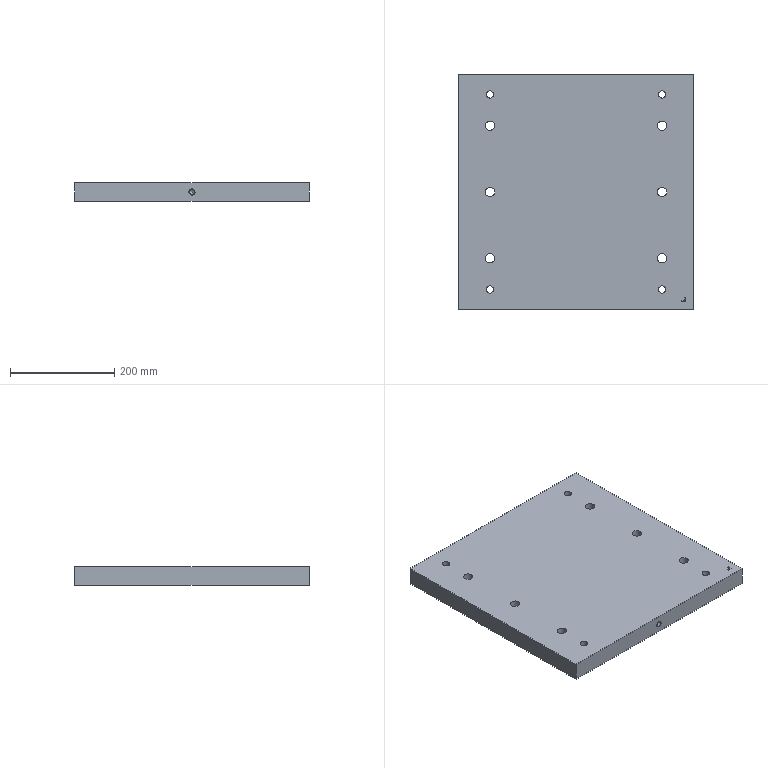Part | NX | features solid 2 | 1 solid | 59 faces | box 450 x 450 x 35 mm | volume 6967341 mm3 | plane 31 | cylinder 26 | cone 2 | commonest cylinder face diameters 18 x6 26 x6 14 x4 20 x4 10.2 x2 11.7 x2
STEP:
#1=CARTESIAN_POINT('',(0.,225.,-392.9));
#2=VERTEX_POINT('',#1);
#3=CARTESIAN_POINT('',(0.,225.,-398.));
#4=DIRECTION('',(0.,1.,0.));
#5=DIRECTION('',(0.,0.,1.));
#6=AXIS2_PLACEMENT_3D('',#3,#4,#5);
#7=CIRCLE('',#6,5.1);
#8=EDGE_CURVE('',#2,#2,#7,.T.);
#9=ORIENTED_EDGE('',*,*,#8,.F.);
#10=EDGE_LOOP('',(#9));
#11=FACE_BOUND('',#10,.T.);
#12=CARTESIAN_POINT('',(-225.,225.,-415.5));
#13=VERTEX_POINT('',#12);
#14=CARTESIAN_POINT('',(-225.,225.,-380.5));
#15=VERTEX_POINT('',#14);
#16=CARTESIAN_POINT('',(-225.,225.,-415.5));
#17=DIRECTION('',(0.,0.,1.));
#18=VECTOR('',#17,1000.);
#19=LINE('',#16,#18);
#20=EDGE_CURVE('',#13,#15,#19,.T.);
#21=ORIENTED_EDGE('',*,*,#20,.T.);
#22=CARTESIAN_POINT('',(225.,225.,-380.5));
#23=VERTEX_POINT('',#22);
#24=CARTESIAN_POINT('',(0.,225.,-380.5));
#25=DIRECTION('',(1.,0.,0.));
#26=VECTOR('',#25,1000.);
#27=LINE('',#24,#26);
#28=EDGE_CURVE('',#15,#23,#27,.T.);
#29=ORIENTED_EDGE('',*,*,#28,.T.);
#30=CARTESIAN_POINT('',(225.,225.,-415.5));
#31=VERTEX_POINT('',#30);
#32=CARTESIAN_POINT('',(225.,225.,-415.5));
#33=DIRECTION('',(0.,0.,1.));
#34=VECTOR('',#33,1000.);
#35=LINE('',#32,#34);
#36=EDGE_CURVE('',#31,#23,#35,.T.);
#37=ORIENTED_EDGE('',*,*,#36,.F.);
#38=CARTESIAN_POINT('',(0.,225.,-415.5));
#39=DIRECTION('',(-1.,0.,0.));
#40=VECTOR('',#39,1000.);
#41=LINE('',#38,#40);
#42=EDGE_CURVE('',#31,#13,#41,.T.);
#43=ORIENTED_EDGE('',*,*,#42,.T.);
#44=EDGE_LOOP('',(#21,#29,#37,#43));
#45=FACE_BOUND('',#44,.T.);
#46=CARTESIAN_POINT('',(0.,225.,-403.85));
#47=VERTEX_POINT('',#46);
#48=CARTESIAN_POINT('',(5.85,225.,-398.));
#49=VERTEX_POINT('',#48);
#50=CARTESIAN_POINT('',(0.,225.,-398.));
#51=DIRECTION('',(0.,1.,0.));
#52=DIRECTION('',(0.,0.,1.));
#53=AXIS2_PLACEMENT_3D('',#50,#51,#52);
#54=CIRCLE('',#53,5.85);
#55=EDGE_CURVE('',#47,#49,#54,.T.);
#56=ORIENTED_EDGE('',*,*,#55,.T.);
#57=CARTESIAN_POINT('',(6.,225.,-398.));
#58=VERTEX_POINT('',#57);
#59=CARTESIAN_POINT('',(0.,225.,-398.));
#60=DIRECTION('',(1.,0.,0.));
#61=VECTOR('',#60,1000.);
#62=LINE('',#59,#61);
#63=EDGE_CURVE('',#49,#58,#62,.T.);
#64=ORIENTED_EDGE('',*,*,#63,.T.);
#65=CARTESIAN_POINT('',(0.,225.,-404.));
#66=VERTEX_POINT('',#65);
#67=CARTESIAN_POINT('',(0.,225.,-398.));
#68=DIRECTION('',(0.,1.,0.));
#69=DIRECTION('',(0.,0.,1.));
#70=AXIS2_PLACEMENT_3D('',#67,#68,#69);
#71=CIRCLE('',#70,6.);
#72=EDGE_CURVE('',#66,#58,#71,.T.);
#73=ORIENTED_EDGE('',*,*,#72,.F.);
#74=CARTESIAN_POINT('',(0.,225.,-415.5));
#75=DIRECTION('',(0.,0.,1.));
#76=VECTOR('',#75,1000.);
#77=LINE('',#74,#76);
#78=EDGE_CURVE('',#66,#47,#77,.T.);
#79=ORIENTED_EDGE('',*,*,#78,.T.);
#80=EDGE_LOOP('',(#56,#64,#73,#79));
#81=FACE_BOUND('',#80,.T.);
#82=CARTESIAN_POINT('',(0.,225.,-415.5));
#83=DIRECTION('',(0.,1.,0.));
#84=DIRECTION('',(0.,0.,1.));
#85=AXIS2_PLACEMENT_3D('',#82,#83,#84);
#86=PLANE('',#85);
#87=ADVANCED_FACE('',(#11,#45,#81),#86,.T.);
#88=CARTESIAN_POINT('',(0.,-225.,-403.1));
#89=VERTEX_POINT('',#88);
#90=CARTESIAN_POINT('',(0.,-225.,-398.));
#91=DIRECTION('',(0.,-1.,0.));
#92=DIRECTION('',(0.,0.,-1.));
#93=AXIS2_PLACEMENT_3D('',#90,#91,#92);
#94=CIRCLE('',#93,5.1);
#95=EDGE_CURVE('',#89,#89,#94,.T.);
#96=ORIENTED_EDGE('',*,*,#95,.F.);
#97=EDGE_LOOP('',(#96));
#98=FACE_BOUND('',#97,.T.);
#99=CARTESIAN_POINT('',(225.,-225.,-415.5));
#100=VERTEX_POINT('',#99);
#101=CARTESIAN_POINT('',(225.,-225.,-380.5));
#102=VERTEX_POINT('',#101);
#103=CARTESIAN_POINT('',(225.,-225.,-415.5));
#104=DIRECTION('',(0.,0.,1.));
#105=VECTOR('',#104,1000.);
#106=LINE('',#103,#105);
#107=EDGE_CURVE('',#100,#102,#106,.T.);
#108=ORIENTED_EDGE('',*,*,#107,.T.);
#109=CARTESIAN_POINT('',(-225.,-225.,-380.5));
#110=VERTEX_POINT('',#109);
#111=CARTESIAN_POINT('',(0.,-225.,-380.5));
#112=DIRECTION('',(-1.,0.,0.));
#113=VECTOR('',#112,1000.);
#114=LINE('',#111,#113);
#115=EDGE_CURVE('',#102,#110,#114,.T.);
#116=ORIENTED_EDGE('',*,*,#115,.T.);
#117=CARTESIAN_POINT('',(-225.,-225.,-415.5));
#118=VERTEX_POINT('',#117);
#119=CARTESIAN_POINT('',(-225.,-225.,-415.5));
#120=DIRECTION('',(0.,0.,1.));
#121=VECTOR('',#120,1000.);
#122=LINE('',#119,#121);
#123=EDGE_CURVE('',#118,#110,#122,.T.);
#124=ORIENTED_EDGE('',*,*,#123,.F.);
#125=CARTESIAN_POINT('',(0.,-225.,-415.5));
#126=DIRECTION('',(1.,0.,0.));
#127=VECTOR('',#126,1000.);
#128=LINE('',#125,#127);
#129=EDGE_CURVE('',#118,#100,#128,.T.);
#130=ORIENTED_EDGE('',*,*,#129,.T.);
#131=EDGE_LOOP('',(#108,#116,#124,#130));
#132=FACE_BOUND('',#131,.T.);
#133=CARTESIAN_POINT('',(0.,-225.,-392.15));
#134=VERTEX_POINT('',#133);
#135=CARTESIAN_POINT('',(5.85,-225.,-398.));
#136=VERTEX_POINT('',#135);
#137=CARTESIAN_POINT('',(0.,-225.,-398.));
#138=DIRECTION('',(0.,-1.,0.));
#139=DIRECTION('',(0.,0.,-1.));
#140=AXIS2_PLACEMENT_3D('',#137,#138,#139);
#141=CIRCLE('',#140,5.85);
#142=EDGE_CURVE('',#134,#136,#141,.T.);
#143=ORIENTED_EDGE('',*,*,#142,.T.);
#144=CARTESIAN_POINT('',(6.,-225.,-398.));
#145=VERTEX_POINT('',#144);
#146=CARTESIAN_POINT('',(0.,-225.,-398.));
#147=DIRECTION('',(1.,0.,0.));
#148=VECTOR('',#147,1000.);
#149=LINE('',#146,#148);
#150=EDGE_CURVE('',#136,#145,#149,.T.);
#151=ORIENTED_EDGE('',*,*,#150,.T.);
#152=CARTESIAN_POINT('',(0.,-225.,-392.));
#153=VERTEX_POINT('',#152);
#154=CARTESIAN_POINT('',(0.,-225.,-398.));
#155=DIRECTION('',(0.,-1.,0.));
#156=DIRECTION('',(0.,0.,-1.));
#157=AXIS2_PLACEMENT_3D('',#154,#155,#156);
#158=CIRCLE('',#157,6.);
#159=EDGE_CURVE('',#153,#145,#158,.T.);
#160=ORIENTED_EDGE('',*,*,#159,.F.);
#161=CARTESIAN_POINT('',(0.,-225.,-415.5));
#162=DIRECTION('',(0.,0.,-1.));
#163=VECTOR('',#162,1000.);
#164=LINE('',#161,#163);
#165=EDGE_CURVE('',#153,#134,#164,.T.);
#166=ORIENTED_EDGE('',*,*,#165,.T.);
#167=EDGE_LOOP('',(#143,#151,#160,#166));
#168=FACE_BOUND('',#167,.T.);
#169=CARTESIAN_POINT('',(0.,-225.,-415.5));
#170=DIRECTION('',(0.,-1.,0.));
#171=DIRECTION('',(0.,0.,-1.));
#172=AXIS2_PLACEMENT_3D('',#169,#170,#171);
#173=PLANE('',#172);
#174=ADVANCED_FACE('',(#98,#132,#168),#173,.T.);
#175=CARTESIAN_POINT('',(-156.,127.,-380.5));
#176=VERTEX_POINT('',#175);
#177=CARTESIAN_POINT('',(-165.,127.,-380.5));
#178=DIRECTION('',(0.,0.,1.));
#179=DIRECTION('',(1.,0.,0.));
#180=AXIS2_PLACEMENT_3D('',#177,#178,#179);
#181=CIRCLE('',#180,9.);
#182=EDGE_CURVE('',#176,#176,#181,.T.);
#183=ORIENTED_EDGE('',*,*,#182,.F.);
#184=EDGE_LOOP('',(#183));
#185=FACE_BOUND('',#184,.T.);
#186=CARTESIAN_POINT('',(-156.,0.,-380.5));
#187=VERTEX_POINT('',#186);
#188=CARTESIAN_POINT('',(-165.,0.,-380.5));
#189=DIRECTION('',(0.,0.,1.));
#190=DIRECTION('',(1.,0.,0.));
#191=AXIS2_PLACEMENT_3D('',#188,#189,#190);
#192=CIRCLE('',#191,9.);
#193=EDGE_CURVE('',#187,#187,#192,.T.);
#194=ORIENTED_EDGE('',*,*,#193,.F.);
#195=EDGE_LOOP('',(#194));
#196=FACE_BOUND('',#195,.T.);
#197=CARTESIAN_POINT('',(-156.,-127.,-380.5));
#198=VERTEX_POINT('',#197);
#199=CARTESIAN_POINT('',(-165.,-127.,-380.5));
#200=DIRECTION('',(0.,0.,1.));
#201=DIRECTION('',(1.,0.,0.));
#202=AXIS2_PLACEMENT_3D('',#199,#200,#201);
#203=CIRCLE('',#202,9.);
#204=EDGE_CURVE('',#198,#198,#203,.T.);
#205=ORIENTED_EDGE('',*,*,#204,.F.);
#206=EDGE_LOOP('',(#205));
#207=FACE_BOUND('',#206,.T.);
#208=CARTESIAN_POINT('',(174.,-127.,-380.5));
#209=VERTEX_POINT('',#208);
#210=CARTESIAN_POINT('',(165.,-127.,-380.5));
#211=DIRECTION('',(0.,0.,1.));
#212=DIRECTION('',(1.,0.,0.));
#213=AXIS2_PLACEMENT_3D('',#210,#211,#212);
#214=CIRCLE('',#213,9.);
#215=EDGE_CURVE('',#209,#209,#214,.T.);
#216=ORIENTED_EDGE('',*,*,#215,.F.);
#217=EDGE_LOOP('',(#216));
#218=FACE_BOUND('',#217,.T.);
#219=CARTESIAN_POINT('',(174.,0.,-380.5));
#220=VERTEX_POINT('',#219);
#221=CARTESIAN_POINT('',(165.,0.,-380.5));
#222=DIRECTION('',(0.,0.,1.));
#223=DIRECTION('',(1.,0.,0.));
#224=AXIS2_PLACEMENT_3D('',#221,#222,#223);
#225=CIRCLE('',#224,9.);
#226=EDGE_CURVE('',#220,#220,#225,.T.);
#227=ORIENTED_EDGE('',*,*,#226,.F.);
#228=EDGE_LOOP('',(#227));
#229=FACE_BOUND('',#228,.T.);
#230=CARTESIAN_POINT('',(174.,127.,-380.5));
#231=VERTEX_POINT('',#230);
#232=CARTESIAN_POINT('',(165.,127.,-380.5));
#233=DIRECTION('',(0.,0.,1.));
#234=DIRECTION('',(1.,0.,0.));
#235=AXIS2_PLACEMENT_3D('',#232,#233,#234);
#236=CIRCLE('',#235,9.);
#237=EDGE_CURVE('',#231,#231,#236,.T.);
#238=ORIENTED_EDGE('',*,*,#237,.F.);
#239=EDGE_LOOP('',(#238));
#240=FACE_BOUND('',#239,.T.);
#241=CARTESIAN_POINT('',(-158.,187.,-380.5));
#242=VERTEX_POINT('',#241);
#243=CARTESIAN_POINT('',(-165.,187.,-380.5));
#244=DIRECTION('',(0.,0.,-1.));
#245=DIRECTION('',(1.,0.,0.));
#246=AXIS2_PLACEMENT_3D('',#243,#244,#245);
#247=CIRCLE('',#246,7.);
#248=EDGE_CURVE('',#242,#242,#247,.T.);
#249=ORIENTED_EDGE('',*,*,#248,.T.);
#250=EDGE_LOOP('',(#249));
#251=FACE_BOUND('',#250,.T.);
#252=CARTESIAN_POINT('',(-158.,-187.,-380.5));
#253=VERTEX_POINT('',#252);
#254=CARTESIAN_POINT('',(-165.,-187.,-380.5));
#255=DIRECTION('',(0.,0.,-1.));
#256=DIRECTION('',(1.,0.,0.));
#257=AXIS2_PLACEMENT_3D('',#254,#255,#256);
#258=CIRCLE('',#257,7.);
#259=EDGE_CURVE('',#253,#253,#258,.T.);
#260=ORIENTED_EDGE('',*,*,#259,.T.);
#261=EDGE_LOOP('',(#260));
#262=FACE_BOUND('',#261,.T.);
#263=CARTESIAN_POINT('',(172.,-187.,-380.5));
#264=VERTEX_POINT('',#263);
#265=CARTESIAN_POINT('',(165.,-187.,-380.5));
#266=DIRECTION('',(0.,0.,-1.));
#267=DIRECTION('',(1.,0.,0.));
#268=AXIS2_PLACEMENT_3D('',#265,#266,#267);
#269=CIRCLE('',#268,7.);
#270=EDGE_CURVE('',#264,#264,#269,.T.);
#271=ORIENTED_EDGE('',*,*,#270,.T.);
#272=EDGE_LOOP('',(#271));
#273=FACE_BOUND('',#272,.T.);
#274=CARTESIAN_POINT('',(172.,187.,-380.5));
#275=VERTEX_POINT('',#274);
#276=CARTESIAN_POINT('',(165.,187.,-380.5));
#277=DIRECTION('',(0.,0.,-1.));
#278=DIRECTION('',(1.,0.,0.));
#279=AXIS2_PLACEMENT_3D('',#276,#277,#278);
#280=CIRCLE('',#279,7.);
#281=EDGE_CURVE('',#275,#275,#280,.T.);
#282=ORIENTED_EDGE('',*,*,#281,.T.);
#283=EDGE_LOOP('',(#282));
#284=FACE_BOUND('',#283,.T.);
#285=CARTESIAN_POINT('',(202.5,-210.5,-380.5));
#286=VERTEX_POINT('',#285);
#287=CARTESIAN_POINT('',(210.5,-210.5,-380.5));
#288=VERTEX_POINT('',#287);
#289=CARTESIAN_POINT('',(202.5,-210.5,-380.5));
#290=DIRECTION('',(1.,0.,0.));
#291=VECTOR('',#290,1000.);
#292=LINE('',#289,#291);
#293=EDGE_CURVE('',#286,#288,#292,.T.);
#294=ORIENTED_EDGE('',*,*,#293,.F.);
#295=CARTESIAN_POINT('',(202.5,-208.1,-380.5));
#296=VERTEX_POINT('',#295);
#297=CARTESIAN_POINT('',(202.5,-210.5,-380.5));
#298=DIRECTION('',(0.,-1.,0.));
#299=VECTOR('',#298,1000.);
#300=LINE('',#297,#299);
#301=EDGE_CURVE('',#296,#286,#300,.T.);
#302=ORIENTED_EDGE('',*,*,#301,.F.);
#303=CARTESIAN_POINT('',(208.1,-208.1,-380.5));
#304=VERTEX_POINT('',#303);
#305=CARTESIAN_POINT('',(202.5,-208.1,-380.5));
#306=DIRECTION('',(-1.,0.,0.));
#307=VECTOR('',#306,1000.);
#308=LINE('',#305,#307);
#309=EDGE_CURVE('',#304,#296,#308,.T.);
#310=ORIENTED_EDGE('',*,*,#309,.F.);
#311=CARTESIAN_POINT('',(208.1,-202.5,-380.5));
#312=VERTEX_POINT('',#311);
#313=CARTESIAN_POINT('',(208.1,-208.1,-380.5));
#314=DIRECTION('',(0.,-1.,0.));
#315=VECTOR('',#314,1000.);
#316=LINE('',#313,#315);
#317=EDGE_CURVE('',#312,#304,#316,.T.);
#318=ORIENTED_EDGE('',*,*,#317,.F.);
#319=CARTESIAN_POINT('',(210.5,-202.5,-380.5));
#320=VERTEX_POINT('',#319);
#321=CARTESIAN_POINT('',(208.1,-202.5,-380.5));
#322=DIRECTION('',(-1.,0.,0.));
#323=VECTOR('',#322,1000.);
#324=LINE('',#321,#323);
#325=EDGE_CURVE('',#320,#312,#324,.T.);
#326=ORIENTED_EDGE('',*,*,#325,.F.);
#327=CARTESIAN_POINT('',(210.5,-202.5,-380.5));
#328=DIRECTION('',(0.,1.,0.));
#329=VECTOR('',#328,1000.);
#330=LINE('',#327,#329);
#331=EDGE_CURVE('',#288,#320,#330,.T.);
#332=ORIENTED_EDGE('',*,*,#331,.F.);
#333=EDGE_LOOP('',(#294,#302,#310,#318,#326,#332));
#334=FACE_BOUND('',#333,.T.);
#335=ORIENTED_EDGE('',*,*,#115,.F.);
#336=CARTESIAN_POINT('',(225.,0.,-380.5));
#337=DIRECTION('',(0.,-1.,0.));
#338=VECTOR('',#337,1000.);
#339=LINE('',#336,#338);
#340=EDGE_CURVE('',#23,#102,#339,.T.);
#341=ORIENTED_EDGE('',*,*,#340,.F.);
#342=ORIENTED_EDGE('',*,*,#28,.F.);
#343=CARTESIAN_POINT('',(-225.,0.,-380.5));
#344=DIRECTION('',(0.,1.,0.));
#345=VECTOR('',#344,1000.);
#346=LINE('',#343,#345);
#347=EDGE_CURVE('',#110,#15,#346,.T.);
#348=ORIENTED_EDGE('',*,*,#347,.F.);
#349=EDGE_LOOP('',(#335,#341,#342,#348));
#350=FACE_BOUND('',#349,.T.);
#351=CARTESIAN_POINT('',(0.,0.,-380.5));
#352=DIRECTION('',(0.,0.,1.));
#353=DIRECTION('',(1.,0.,0.));
#354=AXIS2_PLACEMENT_3D('',#351,#352,#353);
#355=PLANE('',#354);
#356=ADVANCED_FACE('',(#185,#196,#207,#218,#229,#240,#251,#262,#273,#284,#334,#350),#355,.T.);
#357=ORIENTED_EDGE('',*,*,#123,.T.);
#358=ORIENTED_EDGE('',*,*,#347,.T.);
#359=ORIENTED_EDGE('',*,*,#20,.F.);
#360=CARTESIAN_POINT('',(-225.,0.,-415.5));
#361=DIRECTION('',(0.,-1.,0.));
#362=VECTOR('',#361,1000.);
#363=LINE('',#360,#362);
#364=EDGE_CURVE('',#13,#118,#363,.T.);
#365=ORIENTED_EDGE('',*,*,#364,.T.);
#366=EDGE_LOOP('',(#357,#358,#359,#365));
#367=FACE_BOUND('',#366,.T.);
#368=CARTESIAN_POINT('',(-225.,0.,-415.5));
#369=DIRECTION('',(-1.,0.,0.));
#370=DIRECTION('',(0.,0.,1.));
#371=AXIS2_PLACEMENT_3D('',#368,#369,#370);
#372=PLANE('',#371);
#373=ADVANCED_FACE('',(#367),#372,.T.);
#374=CARTESIAN_POINT('',(-152.,127.,-415.5));
#375=VERTEX_POINT('',#374);
#376=CARTESIAN_POINT('',(-165.,127.,-415.5));
#377=DIRECTION('',(0.,0.,1.));
#378=DIRECTION('',(1.,0.,0.));
#379=AXIS2_PLACEMENT_3D('',#376,#377,#378);
#380=CIRCLE('',#379,13.);
#381=EDGE_CURVE('',#375,#375,#380,.T.);
#382=ORIENTED_EDGE('',*,*,#381,.T.);
#383=EDGE_LOOP('',(#382));
#384=FACE_BOUND('',#383,.T.);
#385=CARTESIAN_POINT('',(-152.,0.,-415.5));
#386=VERTEX_POINT('',#385);
#387=CARTESIAN_POINT('',(-165.,0.,-415.5));
#388=DIRECTION('',(0.,0.,1.));
#389=DIRECTION('',(1.,0.,0.));
#390=AXIS2_PLACEMENT_3D('',#387,#388,#389);
#391=CIRCLE('',#390,13.);
#392=EDGE_CURVE('',#386,#386,#391,.T.);
#393=ORIENTED_EDGE('',*,*,#392,.T.);
#394=EDGE_LOOP('',(#393));
#395=FACE_BOUND('',#394,.T.);
#396=CARTESIAN_POINT('',(-152.,-127.,-415.5));
#397=VERTEX_POINT('',#396);
#398=CARTESIAN_POINT('',(-165.,-127.,-415.5));
#399=DIRECTION('',(0.,0.,1.));
#400=DIRECTION('',(1.,0.,0.));
#401=AXIS2_PLACEMENT_3D('',#398,#399,#400);
#402=CIRCLE('',#401,13.);
#403=EDGE_CURVE('',#397,#397,#402,.T.);
#404=ORIENTED_EDGE('',*,*,#403,.T.);
#405=EDGE_LOOP('',(#404));
#406=FACE_BOUND('',#405,.T.);
#407=CARTESIAN_POINT('',(178.,-127.,-415.5));
#408=VERTEX_POINT('',#407);
#409=CARTESIAN_POINT('',(165.,-127.,-415.5));
#410=DIRECTION('',(0.,0.,1.));
#411=DIRECTION('',(1.,0.,0.));
#412=AXIS2_PLACEMENT_3D('',#409,#410,#411);
#413=CIRCLE('',#412,13.);
#414=EDGE_CURVE('',#408,#408,#413,.T.);
#415=ORIENTED_EDGE('',*,*,#414,.T.);
#416=EDGE_LOOP('',(#415));
#417=FACE_BOUND('',#416,.T.);
#418=CARTESIAN_POINT('',(178.,0.,-415.5));
#419=VERTEX_POINT('',#418);
#420=CARTESIAN_POINT('',(165.,0.,-415.5));
#421=DIRECTION('',(0.,0.,1.));
#422=DIRECTION('',(1.,0.,0.));
#423=AXIS2_PLACEMENT_3D('',#420,#421,#422);
#424=CIRCLE('',#423,13.);
#425=EDGE_CURVE('',#419,#419,#424,.T.);
#426=ORIENTED_EDGE('',*,*,#425,.T.);
#427=EDGE_LOOP('',(#426));
#428=FACE_BOUND('',#427,.T.);
#429=CARTESIAN_POINT('',(178.,127.,-415.5));
#430=VERTEX_POINT('',#429);
#431=CARTESIAN_POINT('',(165.,127.,-415.5));
#432=DIRECTION('',(0.,0.,1.));
#433=DIRECTION('',(1.,0.,0.));
#434=AXIS2_PLACEMENT_3D('',#431,#432,#433);
#435=CIRCLE('',#434,13.);
#436=EDGE_CURVE('',#430,#430,#435,.T.);
#437=ORIENTED_EDGE('',*,*,#436,.T.);
#438=EDGE_LOOP('',(#437));
#439=FACE_BOUND('',#438,.T.);
#440=CARTESIAN_POINT('',(-155.,187.,-415.5));
#441=VERTEX_POINT('',#440);
#442=CARTESIAN_POINT('',(-165.,187.,-415.5));
#443=DIRECTION('',(0.,0.,1.));
#444=DIRECTION('',(1.,0.,0.));
#445=AXIS2_PLACEMENT_3D('',#442,#443,#444);
#446=CIRCLE('',#445,10.);
#447=EDGE_CURVE('',#441,#441,#446,.T.);
#448=ORIENTED_EDGE('',*,*,#447,.T.);
#449=EDGE_LOOP('',(#448));
#450=FACE_BOUND('',#449,.T.);
#451=CARTESIAN_POINT('',(-155.,-187.,-415.5));
#452=VERTEX_POINT('',#451);
#453=CARTESIAN_POINT('',(-165.,-187.,-415.5));
#454=DIRECTION('',(0.,0.,1.));
#455=DIRECTION('',(1.,0.,0.));
#456=AXIS2_PLACEMENT_3D('',#453,#454,#455);
#457=CIRCLE('',#456,10.);
#458=EDGE_CURVE('',#452,#452,#457,.T.);
#459=ORIENTED_EDGE('',*,*,#458,.T.);
#460=EDGE_LOOP('',(#459));
#461=FACE_BOUND('',#460,.T.);
#462=CARTESIAN_POINT('',(175.,-187.,-415.5));
#463=VERTEX_POINT('',#462);
#464=CARTESIAN_POINT('',(165.,-187.,-415.5));
#465=DIRECTION('',(0.,0.,1.));
#466=DIRECTION('',(1.,0.,0.));
#467=AXIS2_PLACEMENT_3D('',#464,#465,#466);
#468=CIRCLE('',#467,10.);
#469=EDGE_CURVE('',#463,#463,#468,.T.);
#470=ORIENTED_EDGE('',*,*,#469,.T.);
#471=EDGE_LOOP('',(#470));
#472=FACE_BOUND('',#471,.T.);
#473=CARTESIAN_POINT('',(175.,187.,-415.5));
#474=VERTEX_POINT('',#473);
#475=CARTESIAN_POINT('',(165.,187.,-415.5));
#476=DIRECTION('',(0.,0.,1.));
#477=DIRECTION('',(1.,0.,0.));
#478=AXIS2_PLACEMENT_3D('',#475,#476,#477);
#479=CIRCLE('',#478,10.);
#480=EDGE_CURVE('',#474,#474,#479,.T.);
#481=ORIENTED_EDGE('',*,*,#480,.T.);
#482=EDGE_LOOP('',(#481));
#483=FACE_BOUND('',#482,.T.);
#484=CARTESIAN_POINT('',(225.,0.,-415.5));
#485=DIRECTION('',(0.,1.,0.));
#486=VECTOR('',#485,1000.);
#487=LINE('',#484,#486);
#488=EDGE_CURVE('',#100,#31,#487,.T.);
#489=ORIENTED_EDGE('',*,*,#488,.F.);
#490=ORIENTED_EDGE('',*,*,#129,.F.);
#491=ORIENTED_EDGE('',*,*,#364,.F.);
#492=ORIENTED_EDGE('',*,*,#42,.F.);
#493=EDGE_LOOP('',(#489,#490,#491,#492));
#494=FACE_BOUND('',#493,.T.);
#495=CARTESIAN_POINT('',(0.,0.,-415.5));
#496=DIRECTION('',(0.,0.,-1.));
#497=DIRECTION('',(-1.,0.,0.));
#498=AXIS2_PLACEMENT_3D('',#495,#496,#497);
#499=PLANE('',#498);
#500=ADVANCED_FACE('',(#384,#395,#406,#417,#428,#439,#450,#461,#472,#483,#494),#499,.T.);
#501=ORIENTED_EDGE('',*,*,#488,.T.);
#502=ORIENTED_EDGE('',*,*,#36,.T.);
#503=ORIENTED_EDGE('',*,*,#340,.T.);
#504=ORIENTED_EDGE('',*,*,#107,.F.);
#505=EDGE_LOOP('',(#501,#502,#503,#504));
#506=FACE_BOUND('',#505,.T.);
#507=CARTESIAN_POINT('',(225.,0.,-415.5));
#508=DIRECTION('',(1.,0.,0.));
#509=DIRECTION('',(0.,0.,-1.));
#510=AXIS2_PLACEMENT_3D('',#507,#508,#509);
#511=PLANE('',#510);
#512=ADVANCED_FACE('',(#506),#511,.T.);
#513=ORIENTED_EDGE('',*,*,#293,.T.);
#514=CARTESIAN_POINT('',(210.5,-210.5,-380.8));
#515=VERTEX_POINT('',#514);
#516=CARTESIAN_POINT('',(210.5,-210.5,-380.8));
#517=DIRECTION('',(0.,0.,1.));
#518=VECTOR('',#517,1000.);
#519=LINE('',#516,#518);
#520=EDGE_CURVE('',#515,#288,#519,.T.);
#521=ORIENTED_EDGE('',*,*,#520,.F.);
#522=CARTESIAN_POINT('',(202.5,-210.5,-380.8));
#523=VERTEX_POINT('',#522);
#524=CARTESIAN_POINT('',(202.5,-210.5,-380.8));
#525=DIRECTION('',(1.,0.,0.));
#526=VECTOR('',#525,1000.);
#527=LINE('',#524,#526);
#528=EDGE_CURVE('',#523,#515,#527,.T.);
#529=ORIENTED_EDGE('',*,*,#528,.F.);
#530=CARTESIAN_POINT('',(202.5,-210.5,-380.8));
#531=DIRECTION('',(0.,0.,1.));
#532=VECTOR('',#531,1000.);
#533=LINE('',#530,#532);
#534=EDGE_CURVE('',#523,#286,#533,.T.);
#535=ORIENTED_EDGE('',*,*,#534,.T.);
#536=EDGE_LOOP('',(#513,#521,#529,#535));
#537=FACE_BOUND('',#536,.T.);
#538=CARTESIAN_POINT('',(202.5,-210.5,-380.8));
#539=DIRECTION('',(0.,-1.,0.));
#540=DIRECTION('',(0.,0.,-1.));
#541=AXIS2_PLACEMENT_3D('',#538,#539,#540);
#542=PLANE('',#541);
#543=ADVANCED_FACE('',(#537),#542,.F.);
#544=ORIENTED_EDGE('',*,*,#331,.T.);
#545=CARTESIAN_POINT('',(210.5,-202.5,-380.8));
#546=VERTEX_POINT('',#545);
#547=CARTESIAN_POINT('',(210.5,-202.5,-380.8));
#548=DIRECTION('',(0.,0.,1.));
#549=VECTOR('',#548,1000.);
#550=LINE('',#547,#549);
#551=EDGE_CURVE('',#546,#320,#550,.T.);
#552=ORIENTED_EDGE('',*,*,#551,.F.);
#553=CARTESIAN_POINT('',(210.5,-202.5,-380.8));
#554=DIRECTION('',(0.,1.,0.));
#555=VECTOR('',#554,1000.);
#556=LINE('',#553,#555);
#557=EDGE_CURVE('',#515,#546,#556,.T.);
#558=ORIENTED_EDGE('',*,*,#557,.F.);
#559=ORIENTED_EDGE('',*,*,#520,.T.);
#560=EDGE_LOOP('',(#544,#552,#558,#559));
#561=FACE_BOUND('',#560,.T.);
#562=CARTESIAN_POINT('',(210.5,-202.5,-380.8));
#563=DIRECTION('',(1.,0.,0.));
#564=DIRECTION('',(0.,0.,-1.));
#565=AXIS2_PLACEMENT_3D('',#562,#563,#564);
#566=PLANE('',#565);
#567=ADVANCED_FACE('',(#561),#566,.F.);
#568=ORIENTED_EDGE('',*,*,#325,.T.);
#569=CARTESIAN_POINT('',(208.1,-202.5,-380.8));
#570=VERTEX_POINT('',#569);
#571=CARTESIAN_POINT('',(208.1,-202.5,-380.8));
#572=DIRECTION('',(0.,0.,1.));
#573=VECTOR('',#572,1000.);
#574=LINE('',#571,#573);
#575=EDGE_CURVE('',#570,#312,#574,.T.);
#576=ORIENTED_EDGE('',*,*,#575,.F.);
#577=CARTESIAN_POINT('',(208.1,-202.5,-380.8));
#578=DIRECTION('',(-1.,0.,0.));
#579=VECTOR('',#578,1000.);
#580=LINE('',#577,#579);
#581=EDGE_CURVE('',#546,#570,#580,.T.);
#582=ORIENTED_EDGE('',*,*,#581,.F.);
#583=ORIENTED_EDGE('',*,*,#551,.T.);
#584=EDGE_LOOP('',(#568,#576,#582,#583));
#585=FACE_BOUND('',#584,.T.);
#586=CARTESIAN_POINT('',(208.1,-202.5,-380.8));
#587=DIRECTION('',(0.,1.,0.));
#588=DIRECTION('',(0.,0.,1.));
#589=AXIS2_PLACEMENT_3D('',#586,#587,#588);
#590=PLANE('',#589);
#591=ADVANCED_FACE('',(#585),#590,.F.);
#592=ORIENTED_EDGE('',*,*,#317,.T.);
#593=CARTESIAN_POINT('',(208.1,-208.1,-380.8));
#594=VERTEX_POINT('',#593);
#595=CARTESIAN_POINT('',(208.1,-208.1,-380.8));
#596=DIRECTION('',(0.,0.,1.));
#597=VECTOR('',#596,1000.);
#598=LINE('',#595,#597);
#599=EDGE_CURVE('',#594,#304,#598,.T.);
#600=ORIENTED_EDGE('',*,*,#599,.F.);
#601=CARTESIAN_POINT('',(208.1,-208.1,-380.8));
#602=DIRECTION('',(0.,-1.,0.));
#603=VECTOR('',#602,1000.);
#604=LINE('',#601,#603);
#605=EDGE_CURVE('',#570,#594,#604,.T.);
#606=ORIENTED_EDGE('',*,*,#605,.F.);
#607=ORIENTED_EDGE('',*,*,#575,.T.);
#608=EDGE_LOOP('',(#592,#600,#606,#607));
#609=FACE_BOUND('',#608,.T.);
#610=CARTESIAN_POINT('',(208.1,-208.1,-380.8));
#611=DIRECTION('',(-1.,0.,0.));
#612=DIRECTION('',(0.,0.,1.));
#613=AXIS2_PLACEMENT_3D('',#610,#611,#612);
#614=PLANE('',#613);
#615=ADVANCED_FACE('',(#609),#614,.F.);
#616=ORIENTED_EDGE('',*,*,#309,.T.);
#617=CARTESIAN_POINT('',(202.5,-208.1,-380.8));
#618=VERTEX_POINT('',#617);
#619=CARTESIAN_POINT('',(202.5,-208.1,-380.8));
#620=DIRECTION('',(0.,0.,1.));
#621=VECTOR('',#620,1000.);
#622=LINE('',#619,#621);
#623=EDGE_CURVE('',#618,#296,#622,.T.);
#624=ORIENTED_EDGE('',*,*,#623,.F.);
#625=CARTESIAN_POINT('',(202.5,-208.1,-380.8));
#626=DIRECTION('',(-1.,0.,0.));
#627=VECTOR('',#626,1000.);
#628=LINE('',#625,#627);
#629=EDGE_CURVE('',#594,#618,#628,.T.);
#630=ORIENTED_EDGE('',*,*,#629,.F.);
#631=ORIENTED_EDGE('',*,*,#599,.T.);
#632=EDGE_LOOP('',(#616,#624,#630,#631));
#633=FACE_BOUND('',#632,.T.);
#634=CARTESIAN_POINT('',(202.5,-208.1,-380.8));
#635=DIRECTION('',(0.,1.,0.));
#636=DIRECTION('',(0.,0.,1.));
#637=AXIS2_PLACEMENT_3D('',#634,#635,#636);
#638=PLANE('',#637);
#639=ADVANCED_FACE('',(#633),#638,.F.);
#640=ORIENTED_EDGE('',*,*,#301,.T.);
#641=ORIENTED_EDGE('',*,*,#534,.F.);
#642=CARTESIAN_POINT('',(202.5,-210.5,-380.8));
#643=DIRECTION('',(0.,-1.,0.));
#644=VECTOR('',#643,1000.);
#645=LINE('',#642,#644);
#646=EDGE_CURVE('',#618,#523,#645,.T.);
#647=ORIENTED_EDGE('',*,*,#646,.F.);
#648=ORIENTED_EDGE('',*,*,#623,.T.);
#649=EDGE_LOOP('',(#640,#641,#647,#648));
#650=FACE_BOUND('',#649,.T.);
#651=CARTESIAN_POINT('',(202.5,-210.5,-380.8));
#652=DIRECTION('',(-1.,0.,0.));
#653=DIRECTION('',(0.,0.,1.));
#654=AXIS2_PLACEMENT_3D('',#651,#652,#653);
#655=PLANE('',#654);
#656=ADVANCED_FACE('',(#650),#655,.F.);
#657=ORIENTED_EDGE('',*,*,#528,.T.);
#658=ORIENTED_EDGE('',*,*,#557,.T.);
#659=ORIENTED_EDGE('',*,*,#581,.T.);
#660=ORIENTED_EDGE('',*,*,#605,.T.);
#661=ORIENTED_EDGE('',*,*,#629,.T.);
#662=ORIENTED_EDGE('',*,*,#646,.T.);
#663=EDGE_LOOP('',(#657,#658,#659,#660,#661,#662));
#664=FACE_BOUND('',#663,.T.);
#665=CARTESIAN_POINT('',(210.5,-210.5,-380.8));
#666=DIRECTION('',(0.,0.,1.));
#667=DIRECTION('',(1.,0.,0.));
#668=AXIS2_PLACEMENT_3D('',#665,#666,#667);
#669=PLANE('',#668);
#670=ADVANCED_FACE('',(#664),#669,.T.);
#671=CARTESIAN_POINT('',(5.1,-201.,-398.));
#672=VERTEX_POINT('',#671);
#673=CARTESIAN_POINT('',(0.,-201.,-392.9));
#674=VERTEX_POINT('',#673);
#675=CARTESIAN_POINT('',(0.,-201.,-398.));
#676=DIRECTION('',(0.,1.,0.));
#677=DIRECTION('',(0.,0.,1.));
#678=AXIS2_PLACEMENT_3D('',#675,#676,#677);
#679=CIRCLE('',#678,5.1);
#680=EDGE_CURVE('',#672,#674,#679,.T.);
#681=ORIENTED_EDGE('',*,*,#680,.T.);
#682=CARTESIAN_POINT('',(0.,-201.,-392.));
#683=VERTEX_POINT('',#682);
#684=CARTESIAN_POINT('',(0.,-201.,-392.));
#685=DIRECTION('',(0.,0.,-1.));
#686=VECTOR('',#685,1000.);
#687=LINE('',#684,#686);
#688=EDGE_CURVE('',#683,#674,#687,.T.);
#689=ORIENTED_EDGE('',*,*,#688,.F.);
#690=CARTESIAN_POINT('',(6.,-201.,-398.));
#691=VERTEX_POINT('',#690);
#692=CARTESIAN_POINT('',(0.,-201.,-398.));
#693=DIRECTION('',(0.,-1.,0.));
#694=DIRECTION('',(1.,0.,0.));
#695=AXIS2_PLACEMENT_3D('',#692,#693,#694);
#696=CIRCLE('',#695,6.);
#697=EDGE_CURVE('',#683,#691,#696,.T.);
#698=ORIENTED_EDGE('',*,*,#697,.T.);
#699=CARTESIAN_POINT('',(6.,-201.,-398.));
#700=DIRECTION('',(1.,0.,0.));
#701=VECTOR('',#700,1000.);
#702=LINE('',#699,#701);
#703=EDGE_CURVE('',#672,#691,#702,.T.);
#704=ORIENTED_EDGE('',*,*,#703,.F.);
#705=EDGE_LOOP('',(#681,#689,#698,#704));
#706=FACE_BOUND('',#705,.T.);
#707=CARTESIAN_POINT('',(0.,-201.,-398.));
#708=DIRECTION('',(0.,1.,0.));
#709=DIRECTION('',(0.,0.,1.));
#710=AXIS2_PLACEMENT_3D('',#707,#708,#709);
#711=PLANE('',#710);
#712=ADVANCED_FACE('',(#706),#711,.F.);
#713=ORIENTED_EDGE('',*,*,#159,.T.);
#714=CARTESIAN_POINT('',(6.,-201.,-398.));
#715=DIRECTION('',(0.,-1.,0.));
#716=VECTOR('',#715,1000.);
#717=LINE('',#714,#716);
#718=EDGE_CURVE('',#145,#691,#717,.F.);
#719=ORIENTED_EDGE('',*,*,#718,.T.);
#720=ORIENTED_EDGE('',*,*,#697,.F.);
#721=CARTESIAN_POINT('',(0.,-201.,-392.));
#722=DIRECTION('',(0.,-1.,0.));
#723=VECTOR('',#722,1000.);
#724=LINE('',#721,#723);
#725=EDGE_CURVE('',#683,#153,#724,.T.);
#726=ORIENTED_EDGE('',*,*,#725,.T.);
#727=EDGE_LOOP('',(#713,#719,#720,#726));
#728=FACE_BOUND('',#727,.T.);
#729=CARTESIAN_POINT('',(0.,-201.,-398.));
#730=DIRECTION('',(0.,-1.,0.));
#731=DIRECTION('',(1.,0.,0.));
#732=AXIS2_PLACEMENT_3D('',#729,#730,#731);
#733=CYLINDRICAL_SURFACE('',#732,6.);
#734=ADVANCED_FACE('',(#728),#733,.F.);
#735=CARTESIAN_POINT('',(5.85,-202.,-398.));
#736=VERTEX_POINT('',#735);
#737=CARTESIAN_POINT('',(5.1,-202.,-398.));
#738=VERTEX_POINT('',#737);
#739=CARTESIAN_POINT('',(0.,-202.,-398.));
#740=DIRECTION('',(-1.,0.,0.));
#741=VECTOR('',#740,1000.);
#742=LINE('',#739,#741);
#743=EDGE_CURVE('',#736,#738,#742,.T.);
#744=ORIENTED_EDGE('',*,*,#743,.F.);
#745=CARTESIAN_POINT('',(0.,-202.,-392.15));
#746=VERTEX_POINT('',#745);
#747=CARTESIAN_POINT('',(0.,-202.,-398.));
#748=DIRECTION('',(0.,-1.,0.));
#749=DIRECTION('',(1.,0.,0.));
#750=AXIS2_PLACEMENT_3D('',#747,#748,#749);
#751=CIRCLE('',#750,5.85);
#752=EDGE_CURVE('',#746,#736,#751,.T.);
#753=ORIENTED_EDGE('',*,*,#752,.F.);
#754=CARTESIAN_POINT('',(0.,-202.,-392.9));
#755=VERTEX_POINT('',#754);
#756=CARTESIAN_POINT('',(0.,-202.,-398.));
#757=DIRECTION('',(0.,0.,1.));
#758=VECTOR('',#757,1000.);
#759=LINE('',#756,#758);
#760=EDGE_CURVE('',#755,#746,#759,.T.);
#761=ORIENTED_EDGE('',*,*,#760,.F.);
#762=CARTESIAN_POINT('',(0.,-202.,-398.));
#763=DIRECTION('',(0.,1.,0.));
#764=DIRECTION('',(0.,0.,1.));
#765=AXIS2_PLACEMENT_3D('',#762,#763,#764);
#766=CIRCLE('',#765,5.1);
#767=EDGE_CURVE('',#738,#755,#766,.T.);
#768=ORIENTED_EDGE('',*,*,#767,.F.);
#769=EDGE_LOOP('',(#744,#753,#761,#768));
#770=FACE_BOUND('',#769,.T.);
#771=CARTESIAN_POINT('',(0.,-202.,-398.));
#772=DIRECTION('',(0.,1.,0.));
#773=DIRECTION('',(0.,0.,1.));
#774=AXIS2_PLACEMENT_3D('',#771,#772,#773);
#775=PLANE('',#774);
#776=ADVANCED_FACE('',(#770),#775,.T.);
#777=CARTESIAN_POINT('',(0.,-202.,-392.15));
#778=DIRECTION('',(0.,-1.,0.));
#779=VECTOR('',#778,1000.);
#780=LINE('',#777,#779);
#781=EDGE_CURVE('',#746,#134,#780,.T.);
#782=ORIENTED_EDGE('',*,*,#781,.F.);
#783=ORIENTED_EDGE('',*,*,#752,.T.);
#784=CARTESIAN_POINT('',(5.85,-202.,-398.));
#785=DIRECTION('',(0.,-1.,0.));
#786=VECTOR('',#785,1000.);
#787=LINE('',#784,#786);
#788=EDGE_CURVE('',#136,#736,#787,.F.);
#789=ORIENTED_EDGE('',*,*,#788,.F.);
#790=ORIENTED_EDGE('',*,*,#142,.F.);
#791=EDGE_LOOP('',(#782,#783,#789,#790));
#792=FACE_BOUND('',#791,.T.);
#793=CARTESIAN_POINT('',(0.,-202.,-398.));
#794=DIRECTION('',(0.,-1.,0.));
#795=DIRECTION('',(1.,0.,0.));
#796=AXIS2_PLACEMENT_3D('',#793,#794,#795);
#797=CYLINDRICAL_SURFACE('',#796,5.85);
#798=ADVANCED_FACE('',(#792),#797,.T.);
#799=ORIENTED_EDGE('',*,*,#788,.T.);
#800=ORIENTED_EDGE('',*,*,#743,.T.);
#801=CARTESIAN_POINT('',(5.1,-194.949,-398.));
#802=DIRECTION('',(0.,-1.,0.));
#803=VECTOR('',#802,1000.);
#804=LINE('',#801,#803);
#805=EDGE_CURVE('',#672,#738,#804,.T.);
#806=ORIENTED_EDGE('',*,*,#805,.F.);
#807=ORIENTED_EDGE('',*,*,#703,.T.);
#808=ORIENTED_EDGE('',*,*,#718,.F.);
#809=ORIENTED_EDGE('',*,*,#150,.F.);
#810=EDGE_LOOP('',(#799,#800,#806,#807,#808,#809));
#811=FACE_BOUND('',#810,.T.);
#812=CARTESIAN_POINT('',(6.,-201.,-398.));
#813=DIRECTION('',(0.,0.,-1.));
#814=DIRECTION('',(0.,1.,0.));
#815=AXIS2_PLACEMENT_3D('',#812,#813,#814);
#816=PLANE('',#815);
#817=ADVANCED_FACE('',(#811),#816,.T.);
#818=ORIENTED_EDGE('',*,*,#725,.F.);
#819=ORIENTED_EDGE('',*,*,#688,.T.);
#820=CARTESIAN_POINT('',(0.,-194.949,-392.9));
#821=DIRECTION('',(0.,-1.,0.));
#822=VECTOR('',#821,1000.);
#823=LINE('',#820,#822);
#824=EDGE_CURVE('',#755,#674,#823,.F.);
#825=ORIENTED_EDGE('',*,*,#824,.F.);
#826=ORIENTED_EDGE('',*,*,#760,.T.);
#827=ORIENTED_EDGE('',*,*,#781,.T.);
#828=ORIENTED_EDGE('',*,*,#165,.F.);
#829=EDGE_LOOP('',(#818,#819,#825,#826,#827,#828));
#830=FACE_BOUND('',#829,.T.);
#831=CARTESIAN_POINT('',(0.,-201.,-392.));
#832=DIRECTION('',(-1.,0.,0.));
#833=DIRECTION('',(0.,0.,1.));
#834=AXIS2_PLACEMENT_3D('',#831,#832,#833);
#835=PLANE('',#834);
#836=ADVANCED_FACE('',(#830),#835,.T.);
#837=ORIENTED_EDGE('',*,*,#95,.T.);
#838=EDGE_LOOP('',(#837));
#839=FACE_BOUND('',#838,.T.);
#840=CARTESIAN_POINT('',(5.1,-194.949,-398.));
#841=VERTEX_POINT('',#840);
#842=CARTESIAN_POINT('',(0.,-194.949,-398.));
#843=DIRECTION('',(0.,1.,0.));
#844=DIRECTION('',(1.,0.,0.));
#845=AXIS2_PLACEMENT_3D('',#842,#843,#844);
#846=CIRCLE('',#845,5.1);
#847=EDGE_CURVE('',#841,#841,#846,.T.);
#848=ORIENTED_EDGE('',*,*,#847,.T.);
#849=EDGE_LOOP('',(#848));
#850=FACE_BOUND('',#849,.T.);
#851=ORIENTED_EDGE('',*,*,#805,.T.);
#852=ORIENTED_EDGE('',*,*,#767,.T.);
#853=ORIENTED_EDGE('',*,*,#824,.T.);
#854=ORIENTED_EDGE('',*,*,#680,.F.);
#855=EDGE_LOOP('',(#851,#852,#853,#854));
#856=FACE_BOUND('',#855,.T.);
#857=CARTESIAN_POINT('',(0.,-194.949,-398.));
#858=DIRECTION('',(0.,-1.,0.));
#859=DIRECTION('',(1.,0.,0.));
#860=AXIS2_PLACEMENT_3D('',#857,#858,#859);
#861=CYLINDRICAL_SURFACE('',#860,5.1);
#862=ADVANCED_FACE('',(#839,#850,#856),#861,.F.);
#863=ORIENTED_EDGE('',*,*,#847,.F.);
#864=EDGE_LOOP('',(#863));
#865=FACE_BOUND('',#864,.T.);
#866=CARTESIAN_POINT('',(0.,-192.005,-398.));
#867=VERTEX_POINT('',#866);
#868=VERTEX_LOOP('',#867);
#869=FACE_BOUND('',#868,.T.);
#870=CARTESIAN_POINT('',(0.,-192.005,-398.));
#871=DIRECTION('',(0.,-1.,0.));
#872=DIRECTION('',(1.,0.,0.));
#873=AXIS2_PLACEMENT_3D('',#870,#871,#872);
#874=CONICAL_SURFACE('',#873,0.,1.047);
#875=ADVANCED_FACE('',(#865,#869),#874,.F.);
#876=CARTESIAN_POINT('',(5.1,201.,-398.));
#877=VERTEX_POINT('',#876);
#878=CARTESIAN_POINT('',(0.,201.,-403.1));
#879=VERTEX_POINT('',#878);
#880=CARTESIAN_POINT('',(0.,201.,-398.));
#881=DIRECTION('',(0.,-1.,0.));
#882=DIRECTION('',(0.,0.,-1.));
#883=AXIS2_PLACEMENT_3D('',#880,#881,#882);
#884=CIRCLE('',#883,5.1);
#885=EDGE_CURVE('',#877,#879,#884,.T.);
#886=ORIENTED_EDGE('',*,*,#885,.T.);
#887=CARTESIAN_POINT('',(0.,201.,-404.));
#888=VERTEX_POINT('',#887);
#889=CARTESIAN_POINT('',(0.,201.,-404.));
#890=DIRECTION('',(0.,0.,1.));
#891=VECTOR('',#890,1000.);
#892=LINE('',#889,#891);
#893=EDGE_CURVE('',#888,#879,#892,.T.);
#894=ORIENTED_EDGE('',*,*,#893,.F.);
#895=CARTESIAN_POINT('',(6.,201.,-398.));
#896=VERTEX_POINT('',#895);
#897=CARTESIAN_POINT('',(0.,201.,-398.));
#898=DIRECTION('',(0.,1.,0.));
#899=DIRECTION('',(1.,0.,0.));
#900=AXIS2_PLACEMENT_3D('',#897,#898,#899);
#901=CIRCLE('',#900,6.);
#902=EDGE_CURVE('',#888,#896,#901,.T.);
#903=ORIENTED_EDGE('',*,*,#902,.T.);
#904=CARTESIAN_POINT('',(6.,201.,-398.));
#905=DIRECTION('',(1.,0.,0.));
#906=VECTOR('',#905,1000.);
#907=LINE('',#904,#906);
#908=EDGE_CURVE('',#877,#896,#907,.T.);
#909=ORIENTED_EDGE('',*,*,#908,.F.);
#910=EDGE_LOOP('',(#886,#894,#903,#909));
#911=FACE_BOUND('',#910,.T.);
#912=CARTESIAN_POINT('',(0.,201.,-398.));
#913=DIRECTION('',(0.,-1.,0.));
#914=DIRECTION('',(0.,0.,-1.));
#915=AXIS2_PLACEMENT_3D('',#912,#913,#914);
#916=PLANE('',#915);
#917=ADVANCED_FACE('',(#911),#916,.F.);
#918=ORIENTED_EDGE('',*,*,#72,.T.);
#919=CARTESIAN_POINT('',(6.,201.,-398.));
#920=DIRECTION('',(0.,1.,0.));
#921=VECTOR('',#920,1000.);
#922=LINE('',#919,#921);
#923=EDGE_CURVE('',#58,#896,#922,.F.);
#924=ORIENTED_EDGE('',*,*,#923,.T.);
#925=ORIENTED_EDGE('',*,*,#902,.F.);
#926=CARTESIAN_POINT('',(0.,201.,-404.));
#927=DIRECTION('',(0.,1.,0.));
#928=VECTOR('',#927,1000.);
#929=LINE('',#926,#928);
#930=EDGE_CURVE('',#888,#66,#929,.T.);
#931=ORIENTED_EDGE('',*,*,#930,.T.);
#932=EDGE_LOOP('',(#918,#924,#925,#931));
#933=FACE_BOUND('',#932,.T.);
#934=CARTESIAN_POINT('',(0.,201.,-398.));
#935=DIRECTION('',(0.,1.,0.));
#936=DIRECTION('',(1.,0.,0.));
#937=AXIS2_PLACEMENT_3D('',#934,#935,#936);
#938=CYLINDRICAL_SURFACE('',#937,6.);
#939=ADVANCED_FACE('',(#933),#938,.F.);
#940=CARTESIAN_POINT('',(5.85,202.,-398.));
#941=VERTEX_POINT('',#940);
#942=CARTESIAN_POINT('',(5.1,202.,-398.));
#943=VERTEX_POINT('',#942);
#944=CARTESIAN_POINT('',(0.,202.,-398.));
#945=DIRECTION('',(-1.,0.,0.));
#946=VECTOR('',#945,1000.);
#947=LINE('',#944,#946);
#948=EDGE_CURVE('',#941,#943,#947,.T.);
#949=ORIENTED_EDGE('',*,*,#948,.F.);
#950=CARTESIAN_POINT('',(0.,202.,-403.85));
#951=VERTEX_POINT('',#950);
#952=CARTESIAN_POINT('',(0.,202.,-398.));
#953=DIRECTION('',(0.,1.,0.));
#954=DIRECTION('',(1.,0.,0.));
#955=AXIS2_PLACEMENT_3D('',#952,#953,#954);
#956=CIRCLE('',#955,5.85);
#957=EDGE_CURVE('',#951,#941,#956,.T.);
#958=ORIENTED_EDGE('',*,*,#957,.F.);
#959=CARTESIAN_POINT('',(0.,202.,-403.1));
#960=VERTEX_POINT('',#959);
#961=CARTESIAN_POINT('',(0.,202.,-398.));
#962=DIRECTION('',(0.,0.,-1.));
#963=VECTOR('',#962,1000.);
#964=LINE('',#961,#963);
#965=EDGE_CURVE('',#960,#951,#964,.T.);
#966=ORIENTED_EDGE('',*,*,#965,.F.);
#967=CARTESIAN_POINT('',(0.,202.,-398.));
#968=DIRECTION('',(0.,-1.,0.));
#969=DIRECTION('',(0.,0.,-1.));
#970=AXIS2_PLACEMENT_3D('',#967,#968,#969);
#971=CIRCLE('',#970,5.1);
#972=EDGE_CURVE('',#943,#960,#971,.T.);
#973=ORIENTED_EDGE('',*,*,#972,.F.);
#974=EDGE_LOOP('',(#949,#958,#966,#973));
#975=FACE_BOUND('',#974,.T.);
#976=CARTESIAN_POINT('',(0.,202.,-398.));
#977=DIRECTION('',(0.,-1.,0.));
#978=DIRECTION('',(0.,0.,-1.));
#979=AXIS2_PLACEMENT_3D('',#976,#977,#978);
#980=PLANE('',#979);
#981=ADVANCED_FACE('',(#975),#980,.T.);
#982=CARTESIAN_POINT('',(0.,202.,-403.85));
#983=DIRECTION('',(0.,1.,0.));
#984=VECTOR('',#983,1000.);
#985=LINE('',#982,#984);
#986=EDGE_CURVE('',#951,#47,#985,.T.);
#987=ORIENTED_EDGE('',*,*,#986,.F.);
#988=ORIENTED_EDGE('',*,*,#957,.T.);
#989=CARTESIAN_POINT('',(5.85,202.,-398.));
#990=DIRECTION('',(0.,1.,0.));
#991=VECTOR('',#990,1000.);
#992=LINE('',#989,#991);
#993=EDGE_CURVE('',#49,#941,#992,.F.);
#994=ORIENTED_EDGE('',*,*,#993,.F.);
#995=ORIENTED_EDGE('',*,*,#55,.F.);
#996=EDGE_LOOP('',(#987,#988,#994,#995));
#997=FACE_BOUND('',#996,.T.);
#998=CARTESIAN_POINT('',(0.,202.,-398.));
#999=DIRECTION('',(0.,1.,0.));
#1000=DIRECTION('',(1.,0.,0.));
#1001=AXIS2_PLACEMENT_3D('',#998,#999,#1000);
#1002=CYLINDRICAL_SURFACE('',#1001,5.85);
#1003=ADVANCED_FACE('',(#997),#1002,.T.);
#1004=ORIENTED_EDGE('',*,*,#993,.T.);
#1005=ORIENTED_EDGE('',*,*,#948,.T.);
#1006=CARTESIAN_POINT('',(5.1,194.949,-398.));
#1007=DIRECTION('',(0.,1.,0.));
#1008=VECTOR('',#1007,1000.);
#1009=LINE('',#1006,#1008);
#1010=EDGE_CURVE('',#877,#943,#1009,.T.);
#1011=ORIENTED_EDGE('',*,*,#1010,.F.);
#1012=ORIENTED_EDGE('',*,*,#908,.T.);
#1013=ORIENTED_EDGE('',*,*,#923,.F.);
#1014=ORIENTED_EDGE('',*,*,#63,.F.);
#1015=EDGE_LOOP('',(#1004,#1005,#1011,#1012,#1013,#1014));
#1016=FACE_BOUND('',#1015,.T.);
#1017=CARTESIAN_POINT('',(6.,201.,-398.));
#1018=DIRECTION('',(0.,0.,1.));
#1019=DIRECTION('',(0.,-1.,0.));
#1020=AXIS2_PLACEMENT_3D('',#1017,#1018,#1019);
#1021=PLANE('',#1020);
#1022=ADVANCED_FACE('',(#1016),#1021,.T.);
#1023=ORIENTED_EDGE('',*,*,#930,.F.);
#1024=ORIENTED_EDGE('',*,*,#893,.T.);
#1025=CARTESIAN_POINT('',(0.,194.949,-403.1));
#1026=DIRECTION('',(0.,1.,0.));
#1027=VECTOR('',#1026,1000.);
#1028=LINE('',#1025,#1027);
#1029=EDGE_CURVE('',#960,#879,#1028,.F.);
#1030=ORIENTED_EDGE('',*,*,#1029,.F.);
#1031=ORIENTED_EDGE('',*,*,#965,.T.);
#1032=ORIENTED_EDGE('',*,*,#986,.T.);
#1033=ORIENTED_EDGE('',*,*,#78,.F.);
#1034=EDGE_LOOP('',(#1023,#1024,#1030,#1031,#1032,#1033));
#1035=FACE_BOUND('',#1034,.T.);
#1036=CARTESIAN_POINT('',(0.,201.,-404.));
#1037=DIRECTION('',(-1.,0.,0.));
#1038=DIRECTION('',(0.,0.,1.));
#1039=AXIS2_PLACEMENT_3D('',#1036,#1037,#1038);
#1040=PLANE('',#1039);
#1041=ADVANCED_FACE('',(#1035),#1040,.T.);
#1042=ORIENTED_EDGE('',*,*,#8,.T.);
#1043=EDGE_LOOP('',(#1042));
#1044=FACE_BOUND('',#1043,.T.);
#1045=CARTESIAN_POINT('',(5.1,194.949,-398.));
#1046=VERTEX_POINT('',#1045);
#1047=CARTESIAN_POINT('',(0.,194.949,-398.));
#1048=DIRECTION('',(0.,-1.,0.));
#1049=DIRECTION('',(1.,0.,0.));
#1050=AXIS2_PLACEMENT_3D('',#1047,#1048,#1049);
#1051=CIRCLE('',#1050,5.1);
#1052=EDGE_CURVE('',#1046,#1046,#1051,.T.);
#1053=ORIENTED_EDGE('',*,*,#1052,.T.);
#1054=EDGE_LOOP('',(#1053));
#1055=FACE_BOUND('',#1054,.T.);
#1056=ORIENTED_EDGE('',*,*,#1010,.T.);
#1057=ORIENTED_EDGE('',*,*,#972,.T.);
#1058=ORIENTED_EDGE('',*,*,#1029,.T.);
#1059=ORIENTED_EDGE('',*,*,#885,.F.);
#1060=EDGE_LOOP('',(#1056,#1057,#1058,#1059));
#1061=FACE_BOUND('',#1060,.T.);
#1062=CARTESIAN_POINT('',(0.,194.949,-398.));
#1063=DIRECTION('',(0.,1.,0.));
#1064=DIRECTION('',(1.,0.,0.));
#1065=AXIS2_PLACEMENT_3D('',#1062,#1063,#1064);
#1066=CYLINDRICAL_SURFACE('',#1065,5.1);
#1067=ADVANCED_FACE('',(#1044,#1055,#1061),#1066,.F.);
#1068=ORIENTED_EDGE('',*,*,#1052,.F.);
#1069=EDGE_LOOP('',(#1068));
#1070=FACE_BOUND('',#1069,.T.);
#1071=CARTESIAN_POINT('',(0.,192.005,-398.));
#1072=VERTEX_POINT('',#1071);
#1073=VERTEX_LOOP('',#1072);
#1074=FACE_BOUND('',#1073,.T.);
#1075=CARTESIAN_POINT('',(0.,192.005,-398.));
#1076=DIRECTION('',(0.,1.,0.));
#1077=DIRECTION('',(1.,0.,0.));
#1078=AXIS2_PLACEMENT_3D('',#1075,#1076,#1077);
#1079=CONICAL_SURFACE('',#1078,0.,1.047);
#1080=ADVANCED_FACE('',(#1070,#1074),#1079,.F.);
#1081=CARTESIAN_POINT('',(165.,180.,-402.5));
#1082=VERTEX_POINT('',#1081);
#1083=CARTESIAN_POINT('',(165.,187.,-402.5));
#1084=DIRECTION('',(0.,0.,1.));
#1085=DIRECTION('',(0.,-1.,0.));
#1086=AXIS2_PLACEMENT_3D('',#1083,#1084,#1085);
#1087=CIRCLE('',#1086,7.);
#1088=EDGE_CURVE('',#1082,#1082,#1087,.F.);
#1089=ORIENTED_EDGE('',*,*,#1088,.T.);
#1090=EDGE_LOOP('',(#1089));
#1091=FACE_BOUND('',#1090,.T.);
#1092=ORIENTED_EDGE('',*,*,#281,.F.);
#1093=EDGE_LOOP('',(#1092));
#1094=FACE_BOUND('',#1093,.T.);
#1095=CARTESIAN_POINT('',(165.,187.,-380.5));
#1096=DIRECTION('',(0.,0.,-1.));
#1097=DIRECTION('',(1.,0.,0.));
#1098=AXIS2_PLACEMENT_3D('',#1095,#1096,#1097);
#1099=CYLINDRICAL_SURFACE('',#1098,7.);
#1100=ADVANCED_FACE('',(#1091,#1094),#1099,.F.);
#1101=ORIENTED_EDGE('',*,*,#1088,.F.);
#1102=EDGE_LOOP('',(#1101));
#1103=FACE_BOUND('',#1102,.T.);
#1104=CARTESIAN_POINT('',(175.,187.,-402.5));
#1105=VERTEX_POINT('',#1104);
#1106=CARTESIAN_POINT('',(165.,187.,-402.5));
#1107=DIRECTION('',(0.,0.,-1.));
#1108=DIRECTION('',(1.,0.,0.));
#1109=AXIS2_PLACEMENT_3D('',#1106,#1107,#1108);
#1110=CIRCLE('',#1109,10.);
#1111=EDGE_CURVE('',#1105,#1105,#1110,.T.);
#1112=ORIENTED_EDGE('',*,*,#1111,.T.);
#1113=EDGE_LOOP('',(#1112));
#1114=FACE_BOUND('',#1113,.T.);
#1115=CARTESIAN_POINT('',(165.,187.,-402.5));
#1116=DIRECTION('',(0.,0.,1.));
#1117=DIRECTION('',(0.,-1.,0.));
#1118=AXIS2_PLACEMENT_3D('',#1115,#1116,#1117);
#1119=PLANE('',#1118);
#1120=ADVANCED_FACE('',(#1103,#1114),#1119,.F.);
#1121=ORIENTED_EDGE('',*,*,#480,.F.);
#1122=EDGE_LOOP('',(#1121));
#1123=FACE_BOUND('',#1122,.T.);
#1124=ORIENTED_EDGE('',*,*,#1111,.F.);
#1125=EDGE_LOOP('',(#1124));
#1126=FACE_BOUND('',#1125,.T.);
#1127=CARTESIAN_POINT('',(165.,187.,-402.5));
#1128=DIRECTION('',(0.,0.,-1.));
#1129=DIRECTION('',(1.,0.,0.));
#1130=AXIS2_PLACEMENT_3D('',#1127,#1128,#1129);
#1131=CYLINDRICAL_SURFACE('',#1130,10.);
#1132=ADVANCED_FACE('',(#1123,#1126),#1131,.F.);
#1133=CARTESIAN_POINT('',(165.,-194.,-402.5));
#1134=VERTEX_POINT('',#1133);
#1135=CARTESIAN_POINT('',(165.,-187.,-402.5));
#1136=DIRECTION('',(0.,0.,1.));
#1137=DIRECTION('',(0.,-1.,0.));
#1138=AXIS2_PLACEMENT_3D('',#1135,#1136,#1137);
#1139=CIRCLE('',#1138,7.);
#1140=EDGE_CURVE('',#1134,#1134,#1139,.F.);
#1141=ORIENTED_EDGE('',*,*,#1140,.T.);
#1142=EDGE_LOOP('',(#1141));
#1143=FACE_BOUND('',#1142,.T.);
#1144=ORIENTED_EDGE('',*,*,#270,.F.);
#1145=EDGE_LOOP('',(#1144));
#1146=FACE_BOUND('',#1145,.T.);
#1147=CARTESIAN_POINT('',(165.,-187.,-380.5));
#1148=DIRECTION('',(0.,0.,-1.));
#1149=DIRECTION('',(1.,0.,0.));
#1150=AXIS2_PLACEMENT_3D('',#1147,#1148,#1149);
#1151=CYLINDRICAL_SURFACE('',#1150,7.);
#1152=ADVANCED_FACE('',(#1143,#1146),#1151,.F.);
#1153=ORIENTED_EDGE('',*,*,#1140,.F.);
#1154=EDGE_LOOP('',(#1153));
#1155=FACE_BOUND('',#1154,.T.);
#1156=CARTESIAN_POINT('',(175.,-187.,-402.5));
#1157=VERTEX_POINT('',#1156);
#1158=CARTESIAN_POINT('',(165.,-187.,-402.5));
#1159=DIRECTION('',(0.,0.,-1.));
#1160=DIRECTION('',(1.,0.,0.));
#1161=AXIS2_PLACEMENT_3D('',#1158,#1159,#1160);
#1162=CIRCLE('',#1161,10.);
#1163=EDGE_CURVE('',#1157,#1157,#1162,.T.);
#1164=ORIENTED_EDGE('',*,*,#1163,.T.);
#1165=EDGE_LOOP('',(#1164));
#1166=FACE_BOUND('',#1165,.T.);
#1167=CARTESIAN_POINT('',(165.,-187.,-402.5));
#1168=DIRECTION('',(0.,0.,1.));
#1169=DIRECTION('',(0.,-1.,0.));
#1170=AXIS2_PLACEMENT_3D('',#1167,#1168,#1169);
#1171=PLANE('',#1170);
#1172=ADVANCED_FACE('',(#1155,#1166),#1171,.F.);
#1173=ORIENTED_EDGE('',*,*,#469,.F.);
#1174=EDGE_LOOP('',(#1173));
#1175=FACE_BOUND('',#1174,.T.);
#1176=ORIENTED_EDGE('',*,*,#1163,.F.);
#1177=EDGE_LOOP('',(#1176));
#1178=FACE_BOUND('',#1177,.T.);
#1179=CARTESIAN_POINT('',(165.,-187.,-402.5));
#1180=DIRECTION('',(0.,0.,-1.));
#1181=DIRECTION('',(1.,0.,0.));
#1182=AXIS2_PLACEMENT_3D('',#1179,#1180,#1181);
#1183=CYLINDRICAL_SURFACE('',#1182,10.);
#1184=ADVANCED_FACE('',(#1175,#1178),#1183,.F.);
#1185=CARTESIAN_POINT('',(-165.,-194.,-402.5));
#1186=VERTEX_POINT('',#1185);
#1187=CARTESIAN_POINT('',(-165.,-187.,-402.5));
#1188=DIRECTION('',(0.,0.,1.));
#1189=DIRECTION('',(0.,-1.,0.));
#1190=AXIS2_PLACEMENT_3D('',#1187,#1188,#1189);
#1191=CIRCLE('',#1190,7.);
#1192=EDGE_CURVE('',#1186,#1186,#1191,.F.);
#1193=ORIENTED_EDGE('',*,*,#1192,.T.);
#1194=EDGE_LOOP('',(#1193));
#1195=FACE_BOUND('',#1194,.T.);
#1196=ORIENTED_EDGE('',*,*,#259,.F.);
#1197=EDGE_LOOP('',(#1196));
#1198=FACE_BOUND('',#1197,.T.);
#1199=CARTESIAN_POINT('',(-165.,-187.,-380.5));
#1200=DIRECTION('',(0.,0.,-1.));
#1201=DIRECTION('',(1.,0.,0.));
#1202=AXIS2_PLACEMENT_3D('',#1199,#1200,#1201);
#1203=CYLINDRICAL_SURFACE('',#1202,7.);
#1204=ADVANCED_FACE('',(#1195,#1198),#1203,.F.);
#1205=ORIENTED_EDGE('',*,*,#1192,.F.);
#1206=EDGE_LOOP('',(#1205));
#1207=FACE_BOUND('',#1206,.T.);
#1208=CARTESIAN_POINT('',(-155.,-187.,-402.5));
#1209=VERTEX_POINT('',#1208);
#1210=CARTESIAN_POINT('',(-165.,-187.,-402.5));
#1211=DIRECTION('',(0.,0.,-1.));
#1212=DIRECTION('',(1.,0.,0.));
#1213=AXIS2_PLACEMENT_3D('',#1210,#1211,#1212);
#1214=CIRCLE('',#1213,10.);
#1215=EDGE_CURVE('',#1209,#1209,#1214,.T.);
#1216=ORIENTED_EDGE('',*,*,#1215,.T.);
#1217=EDGE_LOOP('',(#1216));
#1218=FACE_BOUND('',#1217,.T.);
#1219=CARTESIAN_POINT('',(-165.,-187.,-402.5));
#1220=DIRECTION('',(0.,0.,1.));
#1221=DIRECTION('',(0.,-1.,0.));
#1222=AXIS2_PLACEMENT_3D('',#1219,#1220,#1221);
#1223=PLANE('',#1222);
#1224=ADVANCED_FACE('',(#1207,#1218),#1223,.F.);
#1225=ORIENTED_EDGE('',*,*,#458,.F.);
#1226=EDGE_LOOP('',(#1225));
#1227=FACE_BOUND('',#1226,.T.);
#1228=ORIENTED_EDGE('',*,*,#1215,.F.);
#1229=EDGE_LOOP('',(#1228));
#1230=FACE_BOUND('',#1229,.T.);
#1231=CARTESIAN_POINT('',(-165.,-187.,-402.5));
#1232=DIRECTION('',(0.,0.,-1.));
#1233=DIRECTION('',(1.,0.,0.));
#1234=AXIS2_PLACEMENT_3D('',#1231,#1232,#1233);
#1235=CYLINDRICAL_SURFACE('',#1234,10.);
#1236=ADVANCED_FACE('',(#1227,#1230),#1235,.F.);
#1237=CARTESIAN_POINT('',(-165.,180.,-402.5));
#1238=VERTEX_POINT('',#1237);
#1239=CARTESIAN_POINT('',(-165.,187.,-402.5));
#1240=DIRECTION('',(0.,0.,1.));
#1241=DIRECTION('',(0.,-1.,0.));
#1242=AXIS2_PLACEMENT_3D('',#1239,#1240,#1241);
#1243=CIRCLE('',#1242,7.);
#1244=EDGE_CURVE('',#1238,#1238,#1243,.F.);
#1245=ORIENTED_EDGE('',*,*,#1244,.T.);
#1246=EDGE_LOOP('',(#1245));
#1247=FACE_BOUND('',#1246,.T.);
#1248=ORIENTED_EDGE('',*,*,#248,.F.);
#1249=EDGE_LOOP('',(#1248));
#1250=FACE_BOUND('',#1249,.T.);
#1251=CARTESIAN_POINT('',(-165.,187.,-380.5));
#1252=DIRECTION('',(0.,0.,-1.));
#1253=DIRECTION('',(1.,0.,0.));
#1254=AXIS2_PLACEMENT_3D('',#1251,#1252,#1253);
#1255=CYLINDRICAL_SURFACE('',#1254,7.);
#1256=ADVANCED_FACE('',(#1247,#1250),#1255,.F.);
#1257=ORIENTED_EDGE('',*,*,#1244,.F.);
#1258=EDGE_LOOP('',(#1257));
#1259=FACE_BOUND('',#1258,.T.);
#1260=CARTESIAN_POINT('',(-155.,187.,-402.5));
#1261=VERTEX_POINT('',#1260);
#1262=CARTESIAN_POINT('',(-165.,187.,-402.5));
#1263=DIRECTION('',(0.,0.,-1.));
#1264=DIRECTION('',(1.,0.,0.));
#1265=AXIS2_PLACEMENT_3D('',#1262,#1263,#1264);
#1266=CIRCLE('',#1265,10.);
#1267=EDGE_CURVE('',#1261,#1261,#1266,.T.);
#1268=ORIENTED_EDGE('',*,*,#1267,.T.);
#1269=EDGE_LOOP('',(#1268));
#1270=FACE_BOUND('',#1269,.T.);
#1271=CARTESIAN_POINT('',(-165.,187.,-402.5));
#1272=DIRECTION('',(0.,0.,1.));
#1273=DIRECTION('',(0.,-1.,0.));
#1274=AXIS2_PLACEMENT_3D('',#1271,#1272,#1273);
#1275=PLANE('',#1274);
#1276=ADVANCED_FACE('',(#1259,#1270),#1275,.F.);
#1277=ORIENTED_EDGE('',*,*,#447,.F.);
#1278=EDGE_LOOP('',(#1277));
#1279=FACE_BOUND('',#1278,.T.);
#1280=ORIENTED_EDGE('',*,*,#1267,.F.);
#1281=EDGE_LOOP('',(#1280));
#1282=FACE_BOUND('',#1281,.T.);
#1283=CARTESIAN_POINT('',(-165.,187.,-402.5));
#1284=DIRECTION('',(0.,0.,-1.));
#1285=DIRECTION('',(1.,0.,0.));
#1286=AXIS2_PLACEMENT_3D('',#1283,#1284,#1285);
#1287=CYLINDRICAL_SURFACE('',#1286,10.);
#1288=ADVANCED_FACE('',(#1279,#1282),#1287,.F.);
#1289=ORIENTED_EDGE('',*,*,#237,.T.);
#1290=EDGE_LOOP('',(#1289));
#1291=FACE_BOUND('',#1290,.T.);
#1292=CARTESIAN_POINT('',(165.,118.,-396.5));
#1293=VERTEX_POINT('',#1292);
#1294=CARTESIAN_POINT('',(165.,127.,-396.5));
#1295=DIRECTION('',(0.,0.,1.));
#1296=DIRECTION('',(0.,-1.,0.));
#1297=AXIS2_PLACEMENT_3D('',#1294,#1295,#1296);
#1298=CIRCLE('',#1297,9.);
#1299=EDGE_CURVE('',#1293,#1293,#1298,.F.);
#1300=ORIENTED_EDGE('',*,*,#1299,.T.);
#1301=EDGE_LOOP('',(#1300));
#1302=FACE_BOUND('',#1301,.T.);
#1303=CARTESIAN_POINT('',(165.,127.,-190.5));
#1304=DIRECTION('',(0.,0.,-1.));
#1305=DIRECTION('',(1.,0.,0.));
#1306=AXIS2_PLACEMENT_3D('',#1303,#1304,#1305);
#1307=CYLINDRICAL_SURFACE('',#1306,9.);
#1308=ADVANCED_FACE('',(#1291,#1302),#1307,.F.);
#1309=ORIENTED_EDGE('',*,*,#1299,.F.);
#1310=EDGE_LOOP('',(#1309));
#1311=FACE_BOUND('',#1310,.T.);
#1312=CARTESIAN_POINT('',(178.,127.,-396.5));
#1313=VERTEX_POINT('',#1312);
#1314=CARTESIAN_POINT('',(165.,127.,-396.5));
#1315=DIRECTION('',(0.,0.,-1.));
#1316=DIRECTION('',(1.,0.,0.));
#1317=AXIS2_PLACEMENT_3D('',#1314,#1315,#1316);
#1318=CIRCLE('',#1317,13.);
#1319=EDGE_CURVE('',#1313,#1313,#1318,.T.);
#1320=ORIENTED_EDGE('',*,*,#1319,.T.);
#1321=EDGE_LOOP('',(#1320));
#1322=FACE_BOUND('',#1321,.T.);
#1323=CARTESIAN_POINT('',(165.,127.,-396.5));
#1324=DIRECTION('',(0.,0.,1.));
#1325=DIRECTION('',(0.,-1.,0.));
#1326=AXIS2_PLACEMENT_3D('',#1323,#1324,#1325);
#1327=PLANE('',#1326);
#1328=ADVANCED_FACE('',(#1311,#1322),#1327,.F.);
#1329=ORIENTED_EDGE('',*,*,#436,.F.);
#1330=EDGE_LOOP('',(#1329));
#1331=FACE_BOUND('',#1330,.T.);
#1332=ORIENTED_EDGE('',*,*,#1319,.F.);
#1333=EDGE_LOOP('',(#1332));
#1334=FACE_BOUND('',#1333,.T.);
#1335=CARTESIAN_POINT('',(165.,127.,-396.5));
#1336=DIRECTION('',(0.,0.,-1.));
#1337=DIRECTION('',(1.,0.,0.));
#1338=AXIS2_PLACEMENT_3D('',#1335,#1336,#1337);
#1339=CYLINDRICAL_SURFACE('',#1338,13.);
#1340=ADVANCED_FACE('',(#1331,#1334),#1339,.F.);
#1341=ORIENTED_EDGE('',*,*,#226,.T.);
#1342=EDGE_LOOP('',(#1341));
#1343=FACE_BOUND('',#1342,.T.);
#1344=CARTESIAN_POINT('',(165.,-9.,-396.5));
#1345=VERTEX_POINT('',#1344);
#1346=CARTESIAN_POINT('',(165.,0.,-396.5));
#1347=DIRECTION('',(0.,0.,1.));
#1348=DIRECTION('',(0.,-1.,0.));
#1349=AXIS2_PLACEMENT_3D('',#1346,#1347,#1348);
#1350=CIRCLE('',#1349,9.);
#1351=EDGE_CURVE('',#1345,#1345,#1350,.F.);
#1352=ORIENTED_EDGE('',*,*,#1351,.T.);
#1353=EDGE_LOOP('',(#1352));
#1354=FACE_BOUND('',#1353,.T.);
#1355=CARTESIAN_POINT('',(165.,0.,-190.5));
#1356=DIRECTION('',(0.,0.,-1.));
#1357=DIRECTION('',(1.,0.,0.));
#1358=AXIS2_PLACEMENT_3D('',#1355,#1356,#1357);
#1359=CYLINDRICAL_SURFACE('',#1358,9.);
#1360=ADVANCED_FACE('',(#1343,#1354),#1359,.F.);
#1361=ORIENTED_EDGE('',*,*,#1351,.F.);
#1362=EDGE_LOOP('',(#1361));
#1363=FACE_BOUND('',#1362,.T.);
#1364=CARTESIAN_POINT('',(178.,0.,-396.5));
#1365=VERTEX_POINT('',#1364);
#1366=CARTESIAN_POINT('',(165.,0.,-396.5));
#1367=DIRECTION('',(0.,0.,-1.));
#1368=DIRECTION('',(1.,0.,0.));
#1369=AXIS2_PLACEMENT_3D('',#1366,#1367,#1368);
#1370=CIRCLE('',#1369,13.);
#1371=EDGE_CURVE('',#1365,#1365,#1370,.T.);
#1372=ORIENTED_EDGE('',*,*,#1371,.T.);
#1373=EDGE_LOOP('',(#1372));
#1374=FACE_BOUND('',#1373,.T.);
#1375=CARTESIAN_POINT('',(165.,0.,-396.5));
#1376=DIRECTION('',(0.,0.,1.));
#1377=DIRECTION('',(0.,-1.,0.));
#1378=AXIS2_PLACEMENT_3D('',#1375,#1376,#1377);
#1379=PLANE('',#1378);
#1380=ADVANCED_FACE('',(#1363,#1374),#1379,.F.);
#1381=ORIENTED_EDGE('',*,*,#425,.F.);
#1382=EDGE_LOOP('',(#1381));
#1383=FACE_BOUND('',#1382,.T.);
#1384=ORIENTED_EDGE('',*,*,#1371,.F.);
#1385=EDGE_LOOP('',(#1384));
#1386=FACE_BOUND('',#1385,.T.);
#1387=CARTESIAN_POINT('',(165.,0.,-396.5));
#1388=DIRECTION('',(0.,0.,-1.));
#1389=DIRECTION('',(1.,0.,0.));
#1390=AXIS2_PLACEMENT_3D('',#1387,#1388,#1389);
#1391=CYLINDRICAL_SURFACE('',#1390,13.);
#1392=ADVANCED_FACE('',(#1383,#1386),#1391,.F.);
#1393=ORIENTED_EDGE('',*,*,#215,.T.);
#1394=EDGE_LOOP('',(#1393));
#1395=FACE_BOUND('',#1394,.T.);
#1396=CARTESIAN_POINT('',(165.,-136.,-396.5));
#1397=VERTEX_POINT('',#1396);
#1398=CARTESIAN_POINT('',(165.,-127.,-396.5));
#1399=DIRECTION('',(0.,0.,1.));
#1400=DIRECTION('',(0.,-1.,0.));
#1401=AXIS2_PLACEMENT_3D('',#1398,#1399,#1400);
#1402=CIRCLE('',#1401,9.);
#1403=EDGE_CURVE('',#1397,#1397,#1402,.F.);
#1404=ORIENTED_EDGE('',*,*,#1403,.T.);
#1405=EDGE_LOOP('',(#1404));
#1406=FACE_BOUND('',#1405,.T.);
#1407=CARTESIAN_POINT('',(165.,-127.,-190.5));
#1408=DIRECTION('',(0.,0.,-1.));
#1409=DIRECTION('',(1.,0.,0.));
#1410=AXIS2_PLACEMENT_3D('',#1407,#1408,#1409);
#1411=CYLINDRICAL_SURFACE('',#1410,9.);
#1412=ADVANCED_FACE('',(#1395,#1406),#1411,.F.);
#1413=ORIENTED_EDGE('',*,*,#1403,.F.);
#1414=EDGE_LOOP('',(#1413));
#1415=FACE_BOUND('',#1414,.T.);
#1416=CARTESIAN_POINT('',(178.,-127.,-396.5));
#1417=VERTEX_POINT('',#1416);
#1418=CARTESIAN_POINT('',(165.,-127.,-396.5));
#1419=DIRECTION('',(0.,0.,-1.));
#1420=DIRECTION('',(1.,0.,0.));
#1421=AXIS2_PLACEMENT_3D('',#1418,#1419,#1420);
#1422=CIRCLE('',#1421,13.);
#1423=EDGE_CURVE('',#1417,#1417,#1422,.T.);
#1424=ORIENTED_EDGE('',*,*,#1423,.T.);
#1425=EDGE_LOOP('',(#1424));
#1426=FACE_BOUND('',#1425,.T.);
#1427=CARTESIAN_POINT('',(165.,-127.,-396.5));
#1428=DIRECTION('',(0.,0.,1.));
#1429=DIRECTION('',(0.,-1.,0.));
#1430=AXIS2_PLACEMENT_3D('',#1427,#1428,#1429);
#1431=PLANE('',#1430);
#1432=ADVANCED_FACE('',(#1415,#1426),#1431,.F.);
#1433=ORIENTED_EDGE('',*,*,#414,.F.);
#1434=EDGE_LOOP('',(#1433));
#1435=FACE_BOUND('',#1434,.T.);
#1436=ORIENTED_EDGE('',*,*,#1423,.F.);
#1437=EDGE_LOOP('',(#1436));
#1438=FACE_BOUND('',#1437,.T.);
#1439=CARTESIAN_POINT('',(165.,-127.,-396.5));
#1440=DIRECTION('',(0.,0.,-1.));
#1441=DIRECTION('',(1.,0.,0.));
#1442=AXIS2_PLACEMENT_3D('',#1439,#1440,#1441);
#1443=CYLINDRICAL_SURFACE('',#1442,13.);
#1444=ADVANCED_FACE('',(#1435,#1438),#1443,.F.);
#1445=ORIENTED_EDGE('',*,*,#204,.T.);
#1446=EDGE_LOOP('',(#1445));
#1447=FACE_BOUND('',#1446,.T.);
#1448=CARTESIAN_POINT('',(-165.,-136.,-396.5));
#1449=VERTEX_POINT('',#1448);
#1450=CARTESIAN_POINT('',(-165.,-127.,-396.5));
#1451=DIRECTION('',(0.,0.,1.));
#1452=DIRECTION('',(0.,-1.,0.));
#1453=AXIS2_PLACEMENT_3D('',#1450,#1451,#1452);
#1454=CIRCLE('',#1453,9.);
#1455=EDGE_CURVE('',#1449,#1449,#1454,.F.);
#1456=ORIENTED_EDGE('',*,*,#1455,.T.);
#1457=EDGE_LOOP('',(#1456));
#1458=FACE_BOUND('',#1457,.T.);
#1459=CARTESIAN_POINT('',(-165.,-127.,-190.5));
#1460=DIRECTION('',(0.,0.,-1.));
#1461=DIRECTION('',(1.,0.,0.));
#1462=AXIS2_PLACEMENT_3D('',#1459,#1460,#1461);
#1463=CYLINDRICAL_SURFACE('',#1462,9.);
#1464=ADVANCED_FACE('',(#1447,#1458),#1463,.F.);
#1465=ORIENTED_EDGE('',*,*,#1455,.F.);
#1466=EDGE_LOOP('',(#1465));
#1467=FACE_BOUND('',#1466,.T.);
#1468=CARTESIAN_POINT('',(-152.,-127.,-396.5));
#1469=VERTEX_POINT('',#1468);
#1470=CARTESIAN_POINT('',(-165.,-127.,-396.5));
#1471=DIRECTION('',(0.,0.,-1.));
#1472=DIRECTION('',(1.,0.,0.));
#1473=AXIS2_PLACEMENT_3D('',#1470,#1471,#1472);
#1474=CIRCLE('',#1473,13.);
#1475=EDGE_CURVE('',#1469,#1469,#1474,.T.);
#1476=ORIENTED_EDGE('',*,*,#1475,.T.);
#1477=EDGE_LOOP('',(#1476));
#1478=FACE_BOUND('',#1477,.T.);
#1479=CARTESIAN_POINT('',(-165.,-127.,-396.5));
#1480=DIRECTION('',(0.,0.,1.));
#1481=DIRECTION('',(0.,-1.,0.));
#1482=AXIS2_PLACEMENT_3D('',#1479,#1480,#1481);
#1483=PLANE('',#1482);
#1484=ADVANCED_FACE('',(#1467,#1478),#1483,.F.);
#1485=ORIENTED_EDGE('',*,*,#403,.F.);
#1486=EDGE_LOOP('',(#1485));
#1487=FACE_BOUND('',#1486,.T.);
#1488=ORIENTED_EDGE('',*,*,#1475,.F.);
#1489=EDGE_LOOP('',(#1488));
#1490=FACE_BOUND('',#1489,.T.);
#1491=CARTESIAN_POINT('',(-165.,-127.,-396.5));
#1492=DIRECTION('',(0.,0.,-1.));
#1493=DIRECTION('',(1.,0.,0.));
#1494=AXIS2_PLACEMENT_3D('',#1491,#1492,#1493);
#1495=CYLINDRICAL_SURFACE('',#1494,13.);
#1496=ADVANCED_FACE('',(#1487,#1490),#1495,.F.);
#1497=ORIENTED_EDGE('',*,*,#193,.T.);
#1498=EDGE_LOOP('',(#1497));
#1499=FACE_BOUND('',#1498,.T.);
#1500=CARTESIAN_POINT('',(-165.,-9.,-396.5));
#1501=VERTEX_POINT('',#1500);
#1502=CARTESIAN_POINT('',(-165.,0.,-396.5));
#1503=DIRECTION('',(0.,0.,1.));
#1504=DIRECTION('',(0.,-1.,0.));
#1505=AXIS2_PLACEMENT_3D('',#1502,#1503,#1504);
#1506=CIRCLE('',#1505,9.);
#1507=EDGE_CURVE('',#1501,#1501,#1506,.F.);
#1508=ORIENTED_EDGE('',*,*,#1507,.T.);
#1509=EDGE_LOOP('',(#1508));
#1510=FACE_BOUND('',#1509,.T.);
#1511=CARTESIAN_POINT('',(-165.,0.,-190.5));
#1512=DIRECTION('',(0.,0.,-1.));
#1513=DIRECTION('',(1.,0.,0.));
#1514=AXIS2_PLACEMENT_3D('',#1511,#1512,#1513);
#1515=CYLINDRICAL_SURFACE('',#1514,9.);
#1516=ADVANCED_FACE('',(#1499,#1510),#1515,.F.);
#1517=ORIENTED_EDGE('',*,*,#1507,.F.);
#1518=EDGE_LOOP('',(#1517));
#1519=FACE_BOUND('',#1518,.T.);
#1520=CARTESIAN_POINT('',(-152.,0.,-396.5));
#1521=VERTEX_POINT('',#1520);
#1522=CARTESIAN_POINT('',(-165.,0.,-396.5));
#1523=DIRECTION('',(0.,0.,-1.));
#1524=DIRECTION('',(1.,0.,0.));
#1525=AXIS2_PLACEMENT_3D('',#1522,#1523,#1524);
#1526=CIRCLE('',#1525,13.);
#1527=EDGE_CURVE('',#1521,#1521,#1526,.T.);
#1528=ORIENTED_EDGE('',*,*,#1527,.T.);
#1529=EDGE_LOOP('',(#1528));
#1530=FACE_BOUND('',#1529,.T.);
#1531=CARTESIAN_POINT('',(-165.,0.,-396.5));
#1532=DIRECTION('',(0.,0.,1.));
#1533=DIRECTION('',(0.,-1.,0.));
#1534=AXIS2_PLACEMENT_3D('',#1531,#1532,#1533);
#1535=PLANE('',#1534);
#1536=ADVANCED_FACE('',(#1519,#1530),#1535,.F.);
#1537=ORIENTED_EDGE('',*,*,#392,.F.);
#1538=EDGE_LOOP('',(#1537));
#1539=FACE_BOUND('',#1538,.T.);
#1540=ORIENTED_EDGE('',*,*,#1527,.F.);
#1541=EDGE_LOOP('',(#1540));
#1542=FACE_BOUND('',#1541,.T.);
#1543=CARTESIAN_POINT('',(-165.,0.,-396.5));
#1544=DIRECTION('',(0.,0.,-1.));
#1545=DIRECTION('',(1.,0.,0.));
#1546=AXIS2_PLACEMENT_3D('',#1543,#1544,#1545);
#1547=CYLINDRICAL_SURFACE('',#1546,13.);
#1548=ADVANCED_FACE('',(#1539,#1542),#1547,.F.);
#1549=ORIENTED_EDGE('',*,*,#182,.T.);
#1550=EDGE_LOOP('',(#1549));
#1551=FACE_BOUND('',#1550,.T.);
#1552=CARTESIAN_POINT('',(-165.,118.,-396.5));
#1553=VERTEX_POINT('',#1552);
#1554=CARTESIAN_POINT('',(-165.,127.,-396.5));
#1555=DIRECTION('',(0.,0.,1.));
#1556=DIRECTION('',(0.,-1.,0.));
#1557=AXIS2_PLACEMENT_3D('',#1554,#1555,#1556);
#1558=CIRCLE('',#1557,9.);
#1559=EDGE_CURVE('',#1553,#1553,#1558,.F.);
#1560=ORIENTED_EDGE('',*,*,#1559,.T.);
#1561=EDGE_LOOP('',(#1560));
#1562=FACE_BOUND('',#1561,.T.);
#1563=CARTESIAN_POINT('',(-165.,127.,-190.5));
#1564=DIRECTION('',(0.,0.,-1.));
#1565=DIRECTION('',(1.,0.,0.));
#1566=AXIS2_PLACEMENT_3D('',#1563,#1564,#1565);
#1567=CYLINDRICAL_SURFACE('',#1566,9.);
#1568=ADVANCED_FACE('',(#1551,#1562),#1567,.F.);
#1569=ORIENTED_EDGE('',*,*,#1559,.F.);
#1570=EDGE_LOOP('',(#1569));
#1571=FACE_BOUND('',#1570,.T.);
#1572=CARTESIAN_POINT('',(-152.,127.,-396.5));
#1573=VERTEX_POINT('',#1572);
#1574=CARTESIAN_POINT('',(-165.,127.,-396.5));
#1575=DIRECTION('',(0.,0.,-1.));
#1576=DIRECTION('',(1.,0.,0.));
#1577=AXIS2_PLACEMENT_3D('',#1574,#1575,#1576);
#1578=CIRCLE('',#1577,13.);
#1579=EDGE_CURVE('',#1573,#1573,#1578,.T.);
#1580=ORIENTED_EDGE('',*,*,#1579,.T.);
#1581=EDGE_LOOP('',(#1580));
#1582=FACE_BOUND('',#1581,.T.);
#1583=CARTESIAN_POINT('',(-165.,127.,-396.5));
#1584=DIRECTION('',(0.,0.,1.));
#1585=DIRECTION('',(0.,-1.,0.));
#1586=AXIS2_PLACEMENT_3D('',#1583,#1584,#1585);
#1587=PLANE('',#1586);
#1588=ADVANCED_FACE('',(#1571,#1582),#1587,.F.);
#1589=ORIENTED_EDGE('',*,*,#381,.F.);
#1590=EDGE_LOOP('',(#1589));
#1591=FACE_BOUND('',#1590,.T.);
#1592=ORIENTED_EDGE('',*,*,#1579,.F.);
#1593=EDGE_LOOP('',(#1592));
#1594=FACE_BOUND('',#1593,.T.);
#1595=CARTESIAN_POINT('',(-165.,127.,-396.5));
#1596=DIRECTION('',(0.,0.,-1.));
#1597=DIRECTION('',(1.,0.,0.));
#1598=AXIS2_PLACEMENT_3D('',#1595,#1596,#1597);
#1599=CYLINDRICAL_SURFACE('',#1598,13.);
#1600=ADVANCED_FACE('',(#1591,#1594),#1599,.F.);
#1601=CLOSED_SHELL('',(#87,#174,#356,#373,#500,#512,#543,#567,#591,#615,#639,#656,#670,#712,#734,#776,#798,#817,#836,#862,#875,#917,#939,#981,#1003,#1022,#1041,#1067,#1080,#1100,#1120,#1132,#1152,#1172,#1184,#1204,#1224,#1236,#1256,#1276,#1288,#1308,#1328,#1340,#1360,#1380,#1392,#1412,#1432,#1444,#1464,#1484,#1496,#1516,#1536,#1548,#1568,#1588,#1600));
#1602=MANIFOLD_SOLID_BREP('',#1601);
#1603=(LENGTH_UNIT()NAMED_UNIT(*)SI_UNIT(.MILLI.,.METRE.));
#1604=UNCERTAINTY_MEASURE_WITH_UNIT(LENGTH_MEASURE(0.00001),#1603,'','');
#1605=(NAMED_UNIT(*)PLANE_ANGLE_UNIT()SI_UNIT($,.RADIAN.));
#1606=(NAMED_UNIT(*)SI_UNIT($,.STERADIAN.)SOLID_ANGLE_UNIT());
#1607=(GEOMETRIC_REPRESENTATION_CONTEXT(3)GLOBAL_UNCERTAINTY_ASSIGNED_CONTEXT((#1604))GLOBAL_UNIT_ASSIGNED_CONTEXT((#1603,#1605,#1606))REPRESENTATION_CONTEXT('',''));
#1608=ADVANCED_BREP_SHAPE_REPRESENTATION('',(#1602),#1607);